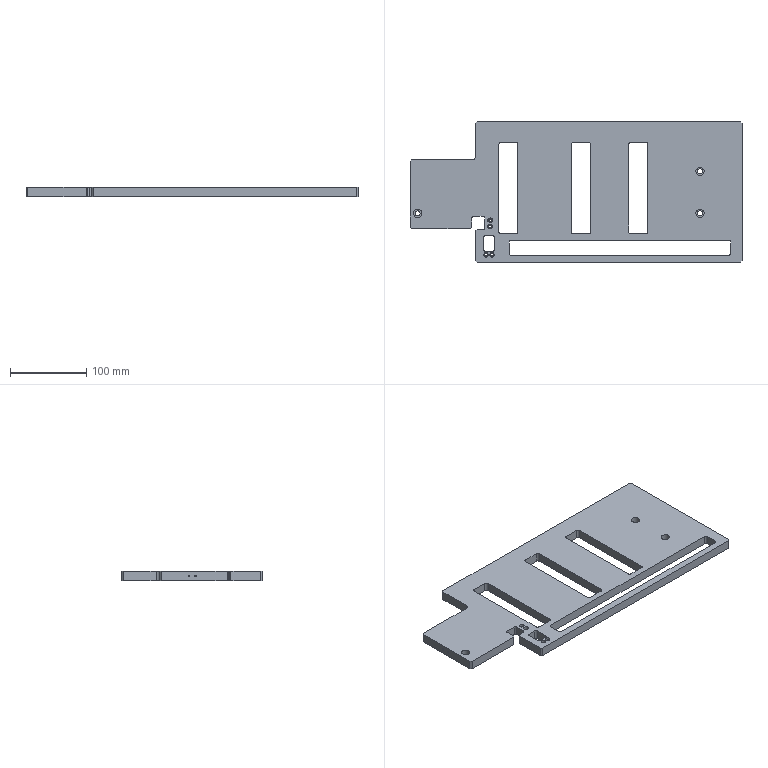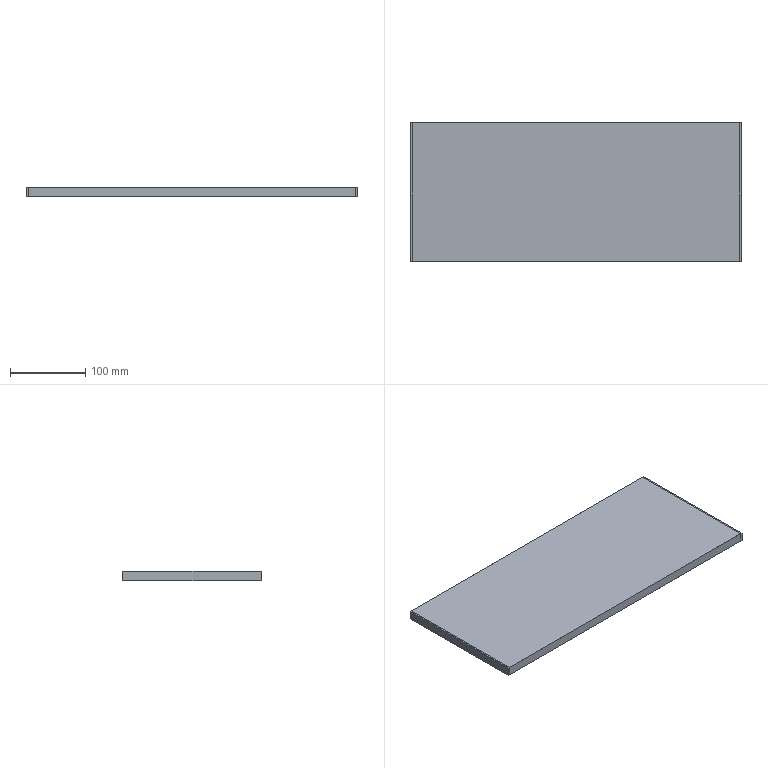CAM job | NX | 3-axis milling, drilling | part box 435 x 184 x 12 mm | stock box 439 x 184 x 12 mm
Tools:
number,name,description,diameter,corner_radius,flute_length,length,flutes
1,D6A45,Milling Tool-5 Parameters,6.0,0.0,50.0,75.0,2
7,3.5ZT,Drilling Tool,3.5,0.0,35.0,50.0,2
16,6.5ZT,Drilling Tool,6.5,0.0,35.0,50.0,2
15,D10,Milling Tool-5 Parameters,10.0,0.0,50.0,75.0,2
14,D10JING,Milling Tool-5 Parameters,10.0,0.0,50.0,75.0,2
12,D6,Milling Tool-5 Parameters,6.0,0.0,50.0,75.0,2
11,D4,Milling Tool-5 Parameters,4.0,0.0,50.0,75.0,2
17,3.3ZT,Drilling Tool,3.2,0.0,35.0,50.0,2
Operations:
program,operation,operation_type,tool,method,geometry_group,spindle_rpm,surface_speed,feed_per_tooth,feed_cut,feed_plunge,cut_length_mm,path_length_mm,cut_time_min,machine_time_min
1,DRILLING_COPY_1,Operation,D6A45,METHOD,A,5000.0,94.0,0.035,350.0,0.0,28.0,617.575,0.08,0.139
1,DRILLING_COPY_1_COPY_COPY_1,Operation,3.5ZT,METHOD,A,2000.0,28.0,0.05,200.0,0.0,68.206,260.203,0.341,0.3602
1,DRILLING_COPY_1_COPY_COPY_1_COPY,Operation,6.5ZT,METHOD,A,2000.0,28.0,0.05,200.0,0.0,53.858,598.811,0.2693,0.3238
1,ZLEVEL_PROFILE_COPY_1_COPY_COPY_1_COPY,ZLevelMilling,D10,METHOD,A,9500.0,298.0,0.1053,2000.0,1000.0,4418.087,7968.208,2.23,2.585
1,ZLEVEL_PROFILE_COPY_1_COPY_COPY_1_COPY_COPY,ZLevelMilling,D10,METHOD,A,9500.0,298.0,0.1579,3000.0,1000.0,2434.441,3286.441,0.84,0.9252
1,ZLEVEL_PROFILE_COPY_1_COPY_COPY_1_COPY_COPY_COPY,ZLevelMilling,D10,METHOD,A,9500.0,298.0,0.1579,3000.0,1000.0,7057.054,7126.054,2.384,2.391
1,ZLEVEL_PROFILE_COPY_1_COPY_COPY_1_COPY_COPY_COPY_COPY,ZLevelMilling,D10,METHOD,A,9500.0,298.0,0.1579,3000.0,1000.0,420.584,489.584,0.172,0.1789
1,ZLEVEL_PROFILE_COPY_1_COPY_COPY_1_COPY_COPY_COPY_COPY_COPY,ZLevelMilling,D10,METHOD,A,9500.0,298.0,0.1579,3000.0,1000.0,397.271,466.271,0.1643,0.1712
1,CAVITY_MILL,CavityMilling,D10,METHOD,A,9500.0,298.0,0.1316,2500.0,1000.0,21123.425,23304.017,9.584,9.802
1,ZLEVEL_PROFILE_COPY_1_COPY_COPY_1_COPY_1,ZLevelMilling,D10JING,METHOD,A,9500.0,298.0,0.0632,1200.0,1000.0,2006.284,3825.579,1.677,1.859
1,HOLE_MILLING,CylinderMilling,D6,METHOD,A,9500.0,179.0,0.0789,1500.0,100.0,825.05,1448.05,0.55,0.6123
1,ZLEVEL_PROFILE_COPY_1_COPY_COPY_1_COPY_COPY_COPY_1,ZLevelMilling,D6,METHOD,A,9500.0,298.0,0.0789,1500.0,1000.0,4602.542,15549.461,3.402,4.497
1,HOLE_MILLING_COPY,CylinderMilling,D4,METHOD,A,9500.0,179.0,0.0789,1500.0,100.0,264.609,568.192,0.1764,0.2068
1,ZLEVEL_PROFILE_COPY_1_COPY_COPY_1_COPY_COPY_COPY_1_COPY,ZLevelMilling,D4,METHOD,A,9500.0,119.0,0.0789,1500.0,1000.0,1982.196,5536.629,1.49,1.846
1,PLANAR_MILL_COPY_COPY_COPY_COPY_COPY_COPY_1_COPY_COPY,PlanarMilling,D6A45,METHOD,A,9500.0,179.0,0.0658,1250.0,100.0,3000.682,4432.738,2.401,2.544
2,DRILLING_COPY_1_COPY,Operation,D6A45,METHOD,B,5000.0,94.0,0.035,350.0,0.0,10.2,153.464,0.0291,0.0435
2,DRILLING_COPY_1_COPY_COPY_1_COPY_1,Operation,3.3ZT,METHOD,B,2785.0,28.0,0.0359,200.0,0.0,33.923,200.91,0.1696,0.1863
2,PLANAR_MILL_COPY_COPY_COPY_COPY_COPY_COPY_1_COPY_COPY_COPY,PlanarMilling,D6A45,METHOD,B,9500.0,179.0,0.0658,1250.0,100.0,2939.82,4699.044,2.352,2.528